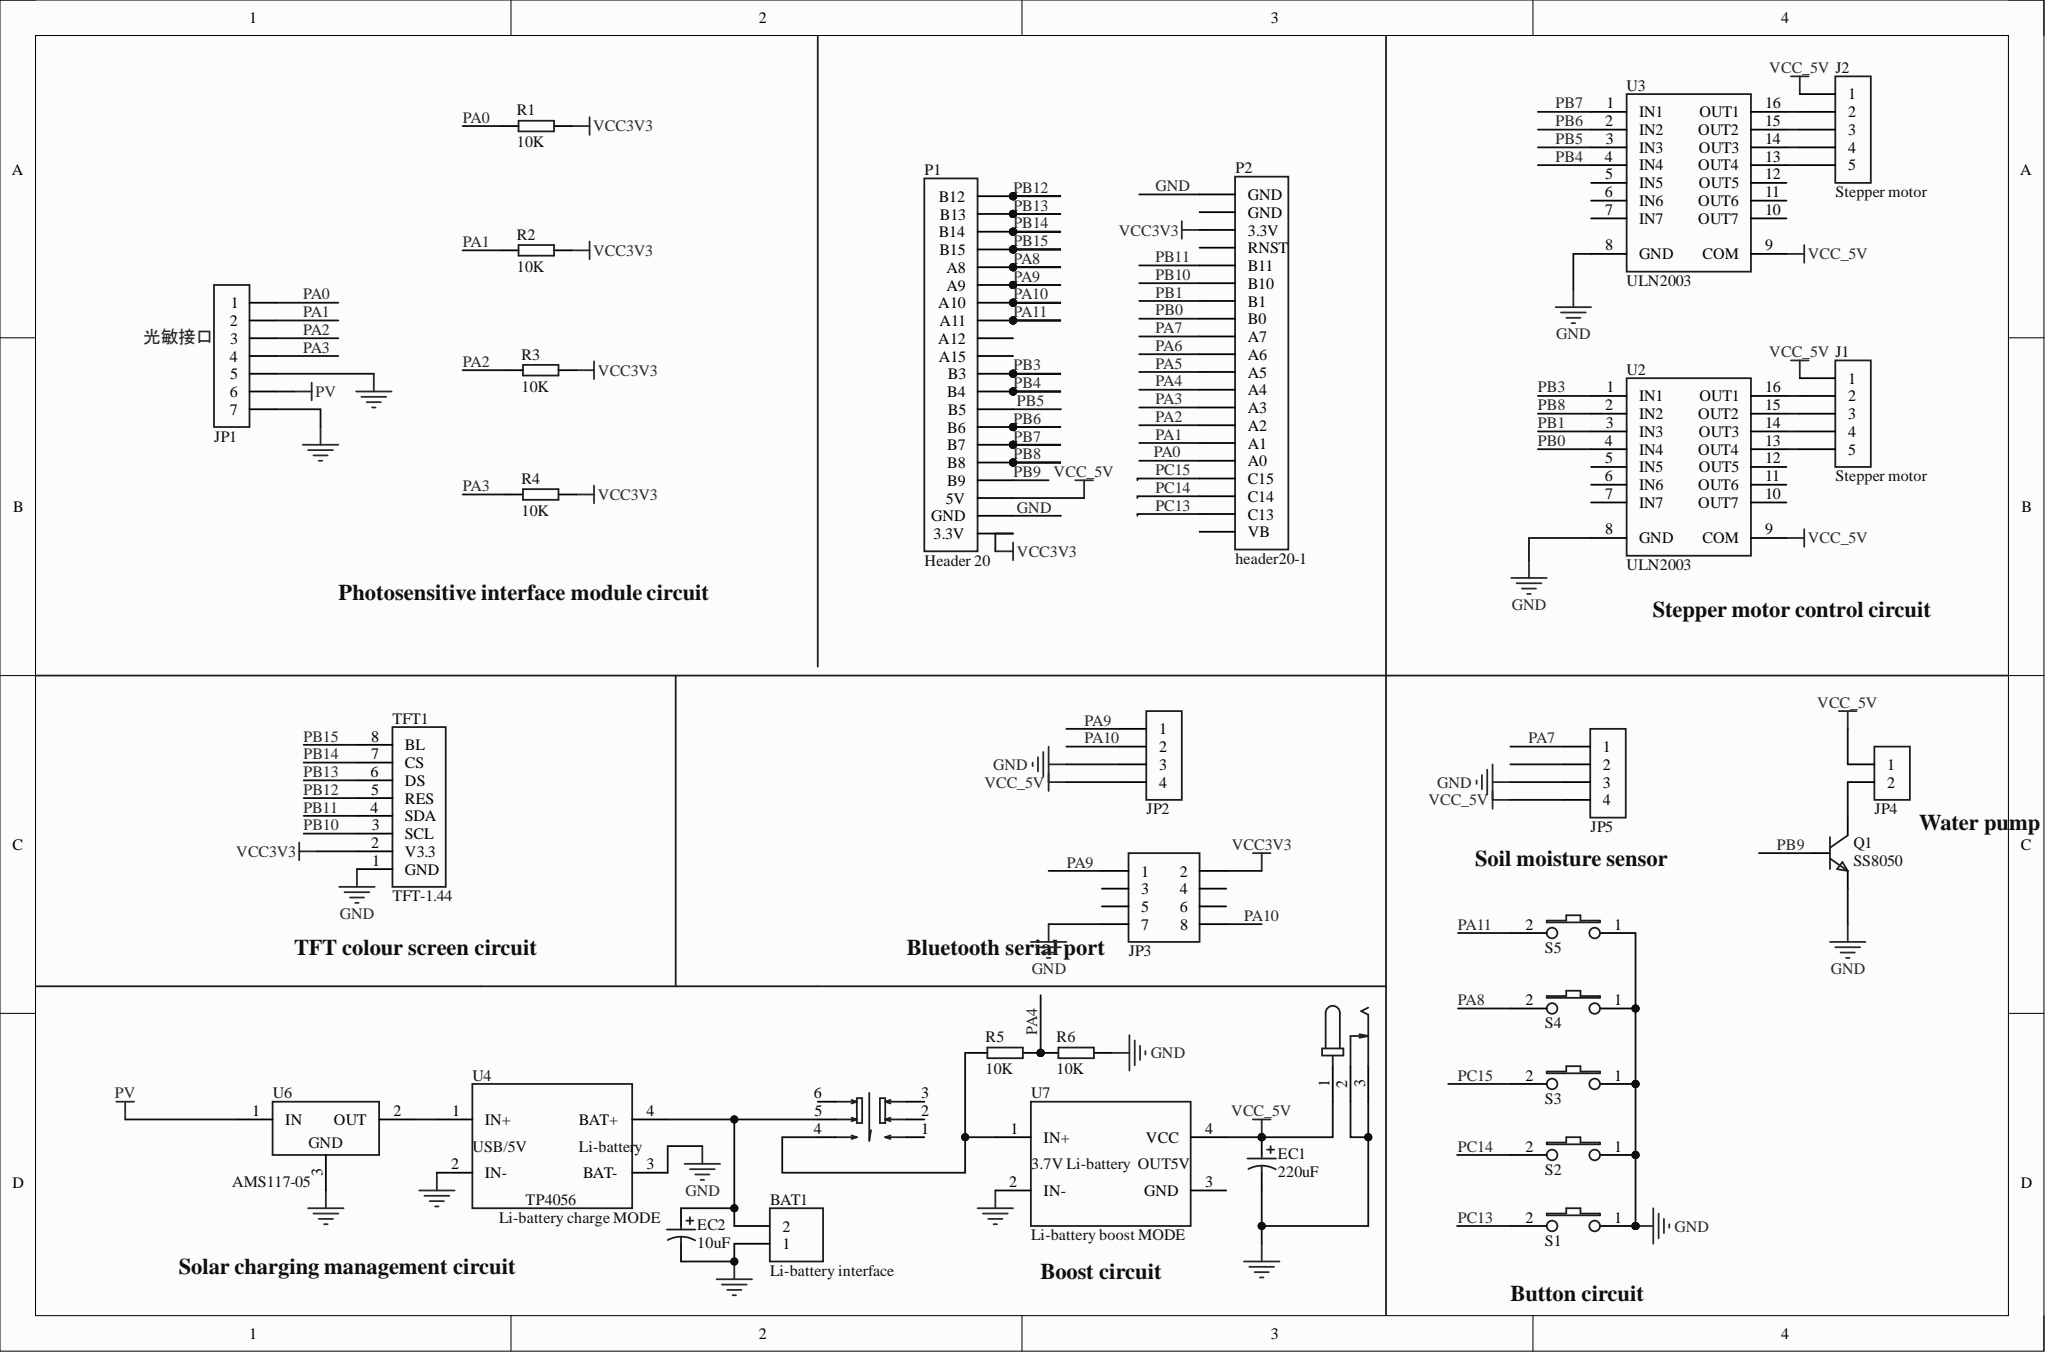Circuit board | Altium Designer | 32 parts | 44 nets
Bill of materials:
Comment,Description,Designator,Footprint,LibRef,Quantity
"Li-battery interface","2-pin terminal block","BAT1","CONN-TH_2P-P5.00_KF301-2P","锂电池接口","1"
"DC002-1.3","","DC1","DC-IN-TH_DC002-1.3","DC002-1.3","1"
"220uF","Polarised capacitor","EC1","CAP-TH_BD10.0-P5.00-D0.6-FD","220uF","1"
"10uF","Polarised capacitor","EC2","CAP-TH_BD5.0-P2.00-D0.8-FD-10UF50VC110GL","10uF","1"
"Stepper motor","Stepper motor interface","J1, J2","CONN-TH_5P-P2.54_C9900008095","步进电机","2"
"HDR-1X7","7P connector","JP1","HDR-TH_7P-P2.54-V-F","HDR-1X7","1"
"HDR-1X4","4P connector","JP2, JP5","HDR-TH_4P-P2.54-V-F","HDR-1X4","2"
"Header 4X2","4*2P connector","JP3","HDR-TH_8P-P2.54-V-F-R2-C4-S2.54-1","Header 4X2","1"
"HDR-1X2","2P connector","JP4","HDR-TH_2P-P2.54-V-F","HDR-1X2","1"
"Header 20","Header, 20-Pin","P1","HDR-TH_20P-P2.54-V-F","Header 20","1"
"header20-1","","P2","HDR-TH_20P-P2.54-V-F","header20-1","1"
"SS8050","High-frequency amplifier, NPN type","Q1","HDR-TH_3P-P2.54-V-F","SS8050","1"
"10K","Resistor","R1, R2, R3, R4, R5, R6","Res_1/8W","10K","6"
"BUTTOM","Button","S1, S2, S3, S4, S5","SW-TH_4P-L6.0-W6.0-P4.50-LS6.5","BUTTOM","5"
"Self-lock button","","SW1","SW-TH_6P-L7.0-W7.0-P2.00","自锁按键","1"
"TFT-1.44","TFT-1.44","TFT1","CONN-TH_8P-P2.50_ZX-XH2.54-8PZZ-GW","TFT-1.44","1"
"ULN2003","ULN2003 chip","U2, U3","PDIP-16_L19.6-W6.5-P2.54-LS7.9-BL","ULN2003","2"
"Li-battery charge MODE","Li-battery charge control module","U4","JYMK","锂电充电MODE","1"
"AMS117-05","7805 regulator chip","U6","CONN-TH_3P-P2.54_8-102202-4","AMS117-05","1"
"Li-battery boost MODE","Li-battery boost module","U7","JYMK","锂电池升压MODE","1"
Netlist (Protel format):
[
BAT1
CONN-TH_2P-P5.00_KF301-2P
Li-battery interface



]
[
DC1
DC-IN-TH_DC002-1.3
DC002-1.3



]
[
EC1
CAP-TH_BD10.0-P5.00-D0.6-FD
220uF



]
[
EC2
CAP-TH_BD5.0-P2.00-D0.8-FD-10UF50VC110GL
10uF



]
[
J1
CONN-TH_5P-P2.54_C9900008095
Stepper motor



]
[
J2
CONN-TH_5P-P2.54_C9900008095
Stepper motor



]
[
JP1
HDR-TH_7P-P2.54-V-F
HDR-1X7



]
[
JP2
HDR-TH_4P-P2.54-V-F
HDR-1X4



]
[
JP3
HDR-TH_8P-P2.54-V-F-R2-C4-S2.54-1
Header 4X2



]
[
JP4
HDR-TH_2P-P2.54-V-F
HDR-1X2



]
[
JP5
HDR-TH_4P-P2.54-V-F
HDR-1X4



]
[
P1
HDR-TH_20P-P2.54-V-F
Header 20



]
[
P2
HDR-TH_20P-P2.54-V-F
header20-1



]
[
Q1
HDR-TH_3P-P2.54-V-F
SS8050



]
[
R1
Res_1/8W
10K



]
[
R2
Res_1/8W
10K



]
[
R3
Res_1/8W
10K



]
[
R4
Res_1/8W
10K



]
[
R5
Res_1/8W
10K



]
[
R6
Res_1/8W
10K



]
[
S1
SW-TH_4P-L6.0-W6.0-P4.50-LS6.5
BUTTOM



]
[
S2
SW-TH_4P-L6.0-W6.0-P4.50-LS6.5
BUTTOM



]
[
S3
SW-TH_4P-L6.0-W6.0-P4.50-LS6.5
BUTTOM



]
[
S4
SW-TH_4P-L6.0-W6.0-P4.50-LS6.5
BUTTOM



]
[
S5
SW-TH_4P-L6.0-W6.0-P4.50-LS6.5
BUTTOM



]
[
SW1
SW-TH_6P-L7.0-W7.0-P2.00
Self-lock button



]
[
TFT1
CONN-TH_8P-P2.50_ZX-XH2.54-8PZZ-GW
TFT-1.44



]
[
U2
PDIP-16_L19.6-W6.5-P2.54-LS7.9-BL
ULN2003



]
[
U3
PDIP-16_L19.6-W6.5-P2.54-LS7.9-BL
ULN2003



]
[
U4
JYMK
Li-battery charge MODE



]
[
U6
CONN-TH_3P-P2.54_8-102202-4
AMS117-05



]
[
U7
JYMK
Li-battery boost MODE



]
(
VCC_5V
DC1-1
EC1-1
J1-1
J2-1
JP2-4
JP4-1
JP5-4
P1-18
U2-9
U3-9
U7-4
)
(
VCC3V3
JP3-2
P1-20
P2-3
R1-2
R2-2
R3-2
R4-2
TFT1-2
)
(
PV
JP1-6
U6-1
)
(
PC15
P2-17
S3-2
)
(
PC14
P2-18
S2-2
)
(
PC13
P2-19
S1-2
)
(
PB15
P1-4
TFT1-8
)
(
PB14
P1-3
TFT1-7
)
(
PB13
P1-2
TFT1-6
)
(
PB12
P1-1
TFT1-5
)
(
PB11
P2-5
TFT1-4
)
(
PB10
P2-6
TFT1-3
)
(
PB9
P1-17
Q1-2
)
(
PB8
P1-16
U2-2
)
(
PB7
P1-15
U3-1
)
(
PB6
P1-14
U3-2
)
(
PB5
P1-13
U3-3
)
(
PB4
P1-12
U3-4
)
(
PB3
P1-11
U2-1
)
(
PB1
P2-7
U2-3
)
(
PB0
P2-8
U2-4
)
(
PA11
P1-8
S5-2
)
(
PA10
JP2-2
JP3-8
P1-7
)
(
PA9
JP2-1
JP3-1
P1-6
)
(
PA8
P1-5
S4-2
)
(
PA7
JP5-1
P2-9
)
(
PA4
P2-12
R5-1
R6-2
)
(
PA3
JP1-4
P2-13
R4-1
)
(
PA2
JP1-3
P2-14
R3-1
)
(
PA1
JP1-2
P2-15
R2-1
)
(
PA0
JP1-1
P2-16
R1-1
)
(
NetU4_1
U4-1
U6-2
)
(
NetR5_2
R5-2
SW1-4
U7-1
)
(
NetJP4_2
JP4-2
Q1-3
)
(
NetJ2_5
J2-5
U3-13
)
(
NetJ2_4
J2-4
U3-14
)
(
NetJ2_3
J2-3
U3-15
)
(
NetJ2_2
J2-2
U3-16
)
(
NetJ1_5
J1-5
U2-13
)
(
NetJ1_4
J1-4
U2-14
)
(
NetJ1_3
J1-3
U2-15
)
(
NetJ1_2
J1-2
U2-16
)
(
NetBAT1_2
BAT1-2
EC2-1
SW1-5
U4-4
)
(
GND
BAT1-1
DC1-2
DC1-3
EC1-2
EC2-2
JP1-5
JP1-7
JP2-3
JP3-7
JP5-3
P1-19
P2-1
Q1-1
R6-1
S1-1
S2-1
S3-1
S4-1
S5-1
TFT1-1
U2-8
U3-8
U4-2
U4-3
U6-3
U7-2
)